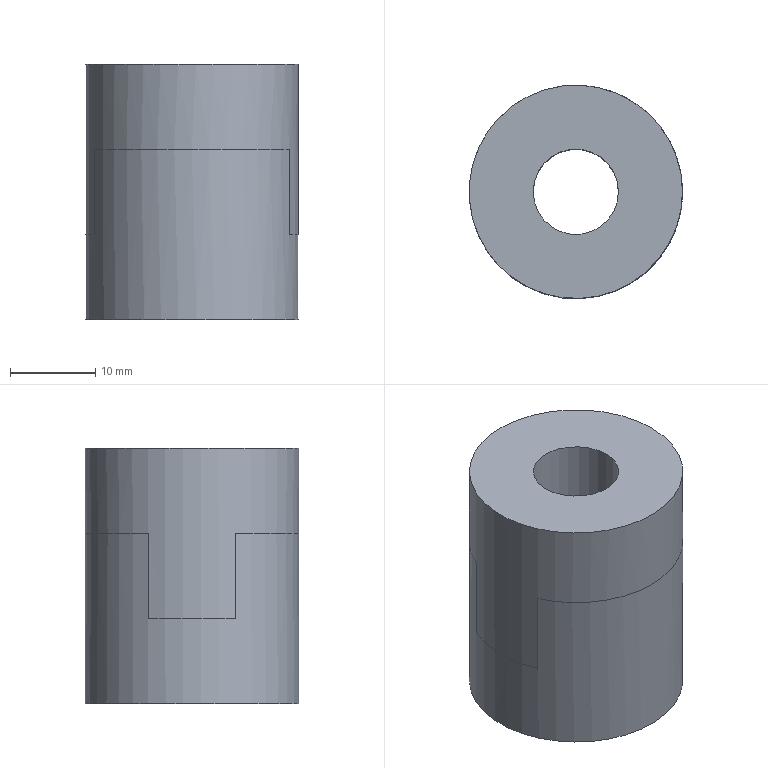Part | NX | features EXTRUDE 6, DATUM_CSYS 4, SKETCH 3 | 2 solids | 16 faces | box 25 x 25 x 30 mm | volume 12370 mm3 | plane 12 | cylinder 4 | commonest cylinder face diameters 10 x2 25 x2
STEP:
#1=CARTESIAN_POINT('',(5.,0.,10.));
#2=VERTEX_POINT('',#1);
#3=CARTESIAN_POINT('',(0.,0.,10.));
#4=DIRECTION('',(0.,0.,1.));
#5=DIRECTION('',(1.,0.,0.));
#6=AXIS2_PLACEMENT_3D('',#3,#4,#5);
#7=CIRCLE('',#6,5.);
#8=EDGE_CURVE('',#2,#2,#7,.T.);
#9=ORIENTED_EDGE('',*,*,#8,.F.);
#10=EDGE_LOOP('',(#9));
#11=FACE_BOUND('',#10,.T.);
#12=CARTESIAN_POINT('',(11.412,-5.1,10.));
#13=VERTEX_POINT('',#12);
#14=CARTESIAN_POINT('',(-11.412,-5.1,10.));
#15=VERTEX_POINT('',#14);
#16=CARTESIAN_POINT('',(11.412,-5.1,10.));
#17=DIRECTION('',(-1.,0.,0.));
#18=VECTOR('',#17,1000.);
#19=LINE('',#16,#18);
#20=EDGE_CURVE('',#13,#15,#19,.T.);
#21=ORIENTED_EDGE('',*,*,#20,.F.);
#22=CARTESIAN_POINT('',(11.412,5.1,10.));
#23=VERTEX_POINT('',#22);
#24=CARTESIAN_POINT('',(0.,0.,10.));
#25=DIRECTION('',(0.,0.,1.));
#26=DIRECTION('',(1.,0.,0.));
#27=AXIS2_PLACEMENT_3D('',#24,#25,#26);
#28=CIRCLE('',#27,12.5);
#29=EDGE_CURVE('',#13,#23,#28,.T.);
#30=ORIENTED_EDGE('',*,*,#29,.T.);
#31=CARTESIAN_POINT('',(-11.412,5.1,10.));
#32=VERTEX_POINT('',#31);
#33=CARTESIAN_POINT('',(-11.412,5.1,10.));
#34=DIRECTION('',(1.,0.,0.));
#35=VECTOR('',#34,1000.);
#36=LINE('',#33,#35);
#37=EDGE_CURVE('',#32,#23,#36,.T.);
#38=ORIENTED_EDGE('',*,*,#37,.F.);
#39=CARTESIAN_POINT('',(0.,0.,10.));
#40=DIRECTION('',(0.,0.,1.));
#41=DIRECTION('',(1.,0.,0.));
#42=AXIS2_PLACEMENT_3D('',#39,#40,#41);
#43=CIRCLE('',#42,12.5);
#44=EDGE_CURVE('',#32,#15,#43,.T.);
#45=ORIENTED_EDGE('',*,*,#44,.T.);
#46=EDGE_LOOP('',(#21,#30,#38,#45));
#47=FACE_BOUND('',#46,.T.);
#48=CARTESIAN_POINT('',(0.,0.,10.));
#49=DIRECTION('',(0.,0.,1.));
#50=DIRECTION('',(1.,0.,0.));
#51=AXIS2_PLACEMENT_3D('',#48,#49,#50);
#52=PLANE('',#51);
#53=ADVANCED_FACE('',(#11,#47),#52,.T.);
#54=ORIENTED_EDGE('',*,*,#44,.F.);
#55=CARTESIAN_POINT('',(-11.412,5.1,20.));
#56=VERTEX_POINT('',#55);
#57=CARTESIAN_POINT('',(-11.412,5.1,20.));
#58=DIRECTION('',(0.,0.,-1.));
#59=VECTOR('',#58,1000.);
#60=LINE('',#57,#59);
#61=EDGE_CURVE('',#32,#56,#60,.F.);
#62=ORIENTED_EDGE('',*,*,#61,.T.);
#63=CARTESIAN_POINT('',(11.412,5.1,20.));
#64=VERTEX_POINT('',#63);
#65=CARTESIAN_POINT('',(0.,0.,20.));
#66=DIRECTION('',(0.,0.,1.));
#67=DIRECTION('',(1.,0.,0.));
#68=AXIS2_PLACEMENT_3D('',#65,#66,#67);
#69=CIRCLE('',#68,12.5);
#70=EDGE_CURVE('',#64,#56,#69,.T.);
#71=ORIENTED_EDGE('',*,*,#70,.F.);
#72=CARTESIAN_POINT('',(11.412,5.1,20.));
#73=DIRECTION('',(0.,0.,-1.));
#74=VECTOR('',#73,1000.);
#75=LINE('',#72,#74);
#76=EDGE_CURVE('',#64,#23,#75,.T.);
#77=ORIENTED_EDGE('',*,*,#76,.T.);
#78=ORIENTED_EDGE('',*,*,#29,.F.);
#79=CARTESIAN_POINT('',(11.412,-5.1,20.));
#80=VERTEX_POINT('',#79);
#81=CARTESIAN_POINT('',(11.412,-5.1,20.));
#82=DIRECTION('',(0.,0.,-1.));
#83=VECTOR('',#82,1000.);
#84=LINE('',#81,#83);
#85=EDGE_CURVE('',#13,#80,#84,.F.);
#86=ORIENTED_EDGE('',*,*,#85,.T.);
#87=CARTESIAN_POINT('',(-11.412,-5.1,20.));
#88=VERTEX_POINT('',#87);
#89=CARTESIAN_POINT('',(0.,0.,20.));
#90=DIRECTION('',(0.,0.,1.));
#91=DIRECTION('',(1.,0.,0.));
#92=AXIS2_PLACEMENT_3D('',#89,#90,#91);
#93=CIRCLE('',#92,12.5);
#94=EDGE_CURVE('',#88,#80,#93,.T.);
#95=ORIENTED_EDGE('',*,*,#94,.F.);
#96=CARTESIAN_POINT('',(-11.412,-5.1,20.));
#97=DIRECTION('',(0.,0.,-1.));
#98=VECTOR('',#97,1000.);
#99=LINE('',#96,#98);
#100=EDGE_CURVE('',#88,#15,#99,.T.);
#101=ORIENTED_EDGE('',*,*,#100,.T.);
#102=EDGE_LOOP('',(#54,#62,#71,#77,#78,#86,#95,#101));
#103=FACE_BOUND('',#102,.T.);
#104=CARTESIAN_POINT('',(12.5,0.,0.));
#105=VERTEX_POINT('',#104);
#106=CARTESIAN_POINT('',(0.,0.,0.));
#107=DIRECTION('',(0.,0.,1.));
#108=DIRECTION('',(1.,0.,0.));
#109=AXIS2_PLACEMENT_3D('',#106,#107,#108);
#110=CIRCLE('',#109,12.5);
#111=EDGE_CURVE('',#105,#105,#110,.T.);
#112=ORIENTED_EDGE('',*,*,#111,.T.);
#113=EDGE_LOOP('',(#112));
#114=FACE_BOUND('',#113,.T.);
#115=CARTESIAN_POINT('',(0.,0.,10.));
#116=DIRECTION('',(0.,0.,-1.));
#117=DIRECTION('',(-1.,0.,0.));
#118=AXIS2_PLACEMENT_3D('',#115,#116,#117);
#119=CYLINDRICAL_SURFACE('',#118,12.5);
#120=ADVANCED_FACE('',(#103,#114),#119,.T.);
#121=CARTESIAN_POINT('',(5.,0.,0.));
#122=VERTEX_POINT('',#121);
#123=CARTESIAN_POINT('',(0.,0.,0.));
#124=DIRECTION('',(0.,0.,1.));
#125=DIRECTION('',(1.,0.,0.));
#126=AXIS2_PLACEMENT_3D('',#123,#124,#125);
#127=CIRCLE('',#126,5.);
#128=EDGE_CURVE('',#122,#122,#127,.T.);
#129=ORIENTED_EDGE('',*,*,#128,.T.);
#130=EDGE_LOOP('',(#129));
#131=FACE_BOUND('',#130,.T.);
#132=ORIENTED_EDGE('',*,*,#111,.F.);
#133=EDGE_LOOP('',(#132));
#134=FACE_BOUND('',#133,.T.);
#135=CARTESIAN_POINT('',(0.,0.,0.));
#136=DIRECTION('',(0.,0.,1.));
#137=DIRECTION('',(1.,0.,0.));
#138=AXIS2_PLACEMENT_3D('',#135,#136,#137);
#139=PLANE('',#138);
#140=ADVANCED_FACE('',(#131,#134),#139,.F.);
#141=ORIENTED_EDGE('',*,*,#37,.T.);
#142=ORIENTED_EDGE('',*,*,#76,.F.);
#143=CARTESIAN_POINT('',(-11.412,5.1,20.));
#144=DIRECTION('',(1.,0.,0.));
#145=VECTOR('',#144,1000.);
#146=LINE('',#143,#145);
#147=EDGE_CURVE('',#56,#64,#146,.T.);
#148=ORIENTED_EDGE('',*,*,#147,.F.);
#149=ORIENTED_EDGE('',*,*,#61,.F.);
#150=EDGE_LOOP('',(#141,#142,#148,#149));
#151=FACE_BOUND('',#150,.T.);
#152=CARTESIAN_POINT('',(-11.412,5.1,20.));
#153=DIRECTION('',(0.,1.,0.));
#154=DIRECTION('',(0.,0.,1.));
#155=AXIS2_PLACEMENT_3D('',#152,#153,#154);
#156=PLANE('',#155);
#157=ADVANCED_FACE('',(#151),#156,.F.);
#158=ORIENTED_EDGE('',*,*,#147,.T.);
#159=ORIENTED_EDGE('',*,*,#70,.T.);
#160=EDGE_LOOP('',(#158,#159));
#161=FACE_BOUND('',#160,.T.);
#162=CARTESIAN_POINT('',(0.,0.,20.));
#163=DIRECTION('',(0.,0.,1.));
#164=DIRECTION('',(1.,0.,0.));
#165=AXIS2_PLACEMENT_3D('',#162,#163,#164);
#166=PLANE('',#165);
#167=ADVANCED_FACE('',(#161),#166,.T.);
#168=ORIENTED_EDGE('',*,*,#20,.T.);
#169=ORIENTED_EDGE('',*,*,#100,.F.);
#170=CARTESIAN_POINT('',(11.412,-5.1,20.));
#171=DIRECTION('',(-1.,0.,0.));
#172=VECTOR('',#171,1000.);
#173=LINE('',#170,#172);
#174=EDGE_CURVE('',#80,#88,#173,.T.);
#175=ORIENTED_EDGE('',*,*,#174,.F.);
#176=ORIENTED_EDGE('',*,*,#85,.F.);
#177=EDGE_LOOP('',(#168,#169,#175,#176));
#178=FACE_BOUND('',#177,.T.);
#179=CARTESIAN_POINT('',(11.412,-5.1,20.));
#180=DIRECTION('',(0.,-1.,0.));
#181=DIRECTION('',(0.,0.,-1.));
#182=AXIS2_PLACEMENT_3D('',#179,#180,#181);
#183=PLANE('',#182);
#184=ADVANCED_FACE('',(#178),#183,.F.);
#185=ORIENTED_EDGE('',*,*,#174,.T.);
#186=ORIENTED_EDGE('',*,*,#94,.T.);
#187=EDGE_LOOP('',(#185,#186));
#188=FACE_BOUND('',#187,.T.);
#189=CARTESIAN_POINT('',(0.,0.,20.));
#190=DIRECTION('',(0.,0.,1.));
#191=DIRECTION('',(1.,0.,0.));
#192=AXIS2_PLACEMENT_3D('',#189,#190,#191);
#193=PLANE('',#192);
#194=ADVANCED_FACE('',(#188),#193,.T.);
#195=ORIENTED_EDGE('',*,*,#8,.T.);
#196=EDGE_LOOP('',(#195));
#197=FACE_BOUND('',#196,.T.);
#198=ORIENTED_EDGE('',*,*,#128,.F.);
#199=EDGE_LOOP('',(#198));
#200=FACE_BOUND('',#199,.T.);
#201=CARTESIAN_POINT('',(0.,0.,-30.));
#202=DIRECTION('',(0.,0.,1.));
#203=DIRECTION('',(1.,0.,0.));
#204=AXIS2_PLACEMENT_3D('',#201,#202,#203);
#205=CYLINDRICAL_SURFACE('',#204,5.);
#206=ADVANCED_FACE('',(#197,#200),#205,.F.);
#207=CLOSED_SHELL('',(#53,#120,#140,#157,#167,#184,#194,#206));
#208=MANIFOLD_SOLID_BREP('',#207);
#209=CARTESIAN_POINT('',(11.412,5.1,10.));
#210=VERTEX_POINT('',#209);
#211=CARTESIAN_POINT('',(-11.412,5.1,10.));
#212=VERTEX_POINT('',#211);
#213=CARTESIAN_POINT('',(11.412,5.1,10.));
#214=DIRECTION('',(-1.,0.,0.));
#215=VECTOR('',#214,1000.);
#216=LINE('',#213,#215);
#217=EDGE_CURVE('',#210,#212,#216,.T.);
#218=ORIENTED_EDGE('',*,*,#217,.T.);
#219=CARTESIAN_POINT('',(-11.412,5.1,20.));
#220=VERTEX_POINT('',#219);
#221=CARTESIAN_POINT('',(-11.412,5.1,20.));
#222=DIRECTION('',(0.,0.,-1.));
#223=VECTOR('',#222,1000.);
#224=LINE('',#221,#223);
#225=EDGE_CURVE('',#212,#220,#224,.F.);
#226=ORIENTED_EDGE('',*,*,#225,.T.);
#227=CARTESIAN_POINT('',(11.412,5.1,20.));
#228=VERTEX_POINT('',#227);
#229=CARTESIAN_POINT('',(11.412,5.1,20.));
#230=DIRECTION('',(-1.,0.,0.));
#231=VECTOR('',#230,1000.);
#232=LINE('',#229,#231);
#233=EDGE_CURVE('',#228,#220,#232,.T.);
#234=ORIENTED_EDGE('',*,*,#233,.F.);
#235=CARTESIAN_POINT('',(11.412,5.1,20.));
#236=DIRECTION('',(0.,0.,-1.));
#237=VECTOR('',#236,1000.);
#238=LINE('',#235,#237);
#239=EDGE_CURVE('',#228,#210,#238,.T.);
#240=ORIENTED_EDGE('',*,*,#239,.T.);
#241=EDGE_LOOP('',(#218,#226,#234,#240));
#242=FACE_BOUND('',#241,.T.);
#243=CARTESIAN_POINT('',(11.412,5.1,20.));
#244=DIRECTION('',(0.,-1.,0.));
#245=DIRECTION('',(0.,0.,-1.));
#246=AXIS2_PLACEMENT_3D('',#243,#244,#245);
#247=PLANE('',#246);
#248=ADVANCED_FACE('',(#242),#247,.F.);
#249=CARTESIAN_POINT('',(-11.412,-5.1,10.));
#250=VERTEX_POINT('',#249);
#251=CARTESIAN_POINT('',(0.,0.,10.));
#252=DIRECTION('',(0.,0.,1.));
#253=DIRECTION('',(1.,0.,0.));
#254=AXIS2_PLACEMENT_3D('',#251,#252,#253);
#255=CIRCLE('',#254,12.5);
#256=EDGE_CURVE('',#212,#250,#255,.T.);
#257=ORIENTED_EDGE('',*,*,#256,.T.);
#258=CARTESIAN_POINT('',(-11.412,-5.1,20.));
#259=VERTEX_POINT('',#258);
#260=CARTESIAN_POINT('',(-11.412,-5.1,20.));
#261=DIRECTION('',(0.,0.,-1.));
#262=VECTOR('',#261,1000.);
#263=LINE('',#260,#262);
#264=EDGE_CURVE('',#250,#259,#263,.F.);
#265=ORIENTED_EDGE('',*,*,#264,.T.);
#266=CARTESIAN_POINT('',(11.412,-5.1,20.));
#267=VERTEX_POINT('',#266);
#268=CARTESIAN_POINT('',(0.,0.,20.));
#269=DIRECTION('',(0.,0.,-1.));
#270=DIRECTION('',(1.,0.,0.));
#271=AXIS2_PLACEMENT_3D('',#268,#269,#270);
#272=CIRCLE('',#271,12.5);
#273=EDGE_CURVE('',#267,#259,#272,.T.);
#274=ORIENTED_EDGE('',*,*,#273,.F.);
#275=CARTESIAN_POINT('',(11.412,-5.1,10.));
#276=VERTEX_POINT('',#275);
#277=CARTESIAN_POINT('',(11.412,-5.1,20.));
#278=DIRECTION('',(0.,0.,-1.));
#279=VECTOR('',#278,1000.);
#280=LINE('',#277,#279);
#281=EDGE_CURVE('',#267,#276,#280,.T.);
#282=ORIENTED_EDGE('',*,*,#281,.T.);
#283=CARTESIAN_POINT('',(0.,0.,10.));
#284=DIRECTION('',(0.,0.,1.));
#285=DIRECTION('',(1.,0.,0.));
#286=AXIS2_PLACEMENT_3D('',#283,#284,#285);
#287=CIRCLE('',#286,12.5);
#288=EDGE_CURVE('',#276,#210,#287,.T.);
#289=ORIENTED_EDGE('',*,*,#288,.T.);
#290=ORIENTED_EDGE('',*,*,#239,.F.);
#291=CARTESIAN_POINT('',(0.,0.,20.));
#292=DIRECTION('',(0.,0.,-1.));
#293=DIRECTION('',(1.,0.,0.));
#294=AXIS2_PLACEMENT_3D('',#291,#292,#293);
#295=CIRCLE('',#294,12.5);
#296=EDGE_CURVE('',#220,#228,#295,.T.);
#297=ORIENTED_EDGE('',*,*,#296,.F.);
#298=ORIENTED_EDGE('',*,*,#225,.F.);
#299=EDGE_LOOP('',(#257,#265,#274,#282,#289,#290,#297,#298));
#300=FACE_BOUND('',#299,.T.);
#301=CARTESIAN_POINT('',(12.5,0.,30.));
#302=VERTEX_POINT('',#301);
#303=CARTESIAN_POINT('',(0.,0.,30.));
#304=DIRECTION('',(0.,0.,-1.));
#305=DIRECTION('',(1.,0.,0.));
#306=AXIS2_PLACEMENT_3D('',#303,#304,#305);
#307=CIRCLE('',#306,12.5);
#308=EDGE_CURVE('',#302,#302,#307,.T.);
#309=ORIENTED_EDGE('',*,*,#308,.T.);
#310=EDGE_LOOP('',(#309));
#311=FACE_BOUND('',#310,.T.);
#312=CARTESIAN_POINT('',(0.,0.,20.));
#313=DIRECTION('',(0.,0.,-1.));
#314=DIRECTION('',(-1.,0.,0.));
#315=AXIS2_PLACEMENT_3D('',#312,#313,#314);
#316=CYLINDRICAL_SURFACE('',#315,12.5);
#317=ADVANCED_FACE('',(#300,#311),#316,.T.);
#318=CARTESIAN_POINT('',(-11.412,-5.1,10.));
#319=DIRECTION('',(1.,0.,0.));
#320=VECTOR('',#319,1000.);
#321=LINE('',#318,#320);
#322=EDGE_CURVE('',#250,#276,#321,.T.);
#323=ORIENTED_EDGE('',*,*,#322,.T.);
#324=ORIENTED_EDGE('',*,*,#281,.F.);
#325=CARTESIAN_POINT('',(-11.412,-5.1,20.));
#326=DIRECTION('',(1.,0.,0.));
#327=VECTOR('',#326,1000.);
#328=LINE('',#325,#327);
#329=EDGE_CURVE('',#259,#267,#328,.T.);
#330=ORIENTED_EDGE('',*,*,#329,.F.);
#331=ORIENTED_EDGE('',*,*,#264,.F.);
#332=EDGE_LOOP('',(#323,#324,#330,#331));
#333=FACE_BOUND('',#332,.T.);
#334=CARTESIAN_POINT('',(-11.412,-5.1,20.));
#335=DIRECTION('',(0.,1.,0.));
#336=DIRECTION('',(0.,0.,1.));
#337=AXIS2_PLACEMENT_3D('',#334,#335,#336);
#338=PLANE('',#337);
#339=ADVANCED_FACE('',(#333),#338,.F.);
#340=CARTESIAN_POINT('',(5.,0.,10.));
#341=VERTEX_POINT('',#340);
#342=CARTESIAN_POINT('',(0.,0.,10.));
#343=DIRECTION('',(0.,0.,1.));
#344=DIRECTION('',(1.,0.,0.));
#345=AXIS2_PLACEMENT_3D('',#342,#343,#344);
#346=CIRCLE('',#345,5.);
#347=EDGE_CURVE('',#341,#341,#346,.T.);
#348=ORIENTED_EDGE('',*,*,#347,.T.);
#349=EDGE_LOOP('',(#348));
#350=FACE_BOUND('',#349,.T.);
#351=ORIENTED_EDGE('',*,*,#288,.F.);
#352=ORIENTED_EDGE('',*,*,#322,.F.);
#353=ORIENTED_EDGE('',*,*,#256,.F.);
#354=ORIENTED_EDGE('',*,*,#217,.F.);
#355=EDGE_LOOP('',(#351,#352,#353,#354));
#356=FACE_BOUND('',#355,.T.);
#357=CARTESIAN_POINT('',(0.,0.,10.));
#358=DIRECTION('',(0.,0.,1.));
#359=DIRECTION('',(1.,0.,0.));
#360=AXIS2_PLACEMENT_3D('',#357,#358,#359);
#361=PLANE('',#360);
#362=ADVANCED_FACE('',(#350,#356),#361,.F.);
#363=ORIENTED_EDGE('',*,*,#296,.T.);
#364=ORIENTED_EDGE('',*,*,#233,.T.);
#365=EDGE_LOOP('',(#363,#364));
#366=FACE_BOUND('',#365,.T.);
#367=CARTESIAN_POINT('',(0.,0.,20.));
#368=DIRECTION('',(0.,0.,-1.));
#369=DIRECTION('',(-1.,0.,0.));
#370=AXIS2_PLACEMENT_3D('',#367,#368,#369);
#371=PLANE('',#370);
#372=ADVANCED_FACE('',(#366),#371,.T.);
#373=CARTESIAN_POINT('',(5.,0.,30.));
#374=VERTEX_POINT('',#373);
#375=CARTESIAN_POINT('',(0.,0.,30.));
#376=DIRECTION('',(0.,0.,1.));
#377=DIRECTION('',(1.,0.,0.));
#378=AXIS2_PLACEMENT_3D('',#375,#376,#377);
#379=CIRCLE('',#378,5.);
#380=EDGE_CURVE('',#374,#374,#379,.T.);
#381=ORIENTED_EDGE('',*,*,#380,.F.);
#382=EDGE_LOOP('',(#381));
#383=FACE_BOUND('',#382,.T.);
#384=ORIENTED_EDGE('',*,*,#308,.F.);
#385=EDGE_LOOP('',(#384));
#386=FACE_BOUND('',#385,.T.);
#387=CARTESIAN_POINT('',(0.,0.,30.));
#388=DIRECTION('',(0.,0.,-1.));
#389=DIRECTION('',(-1.,0.,0.));
#390=AXIS2_PLACEMENT_3D('',#387,#388,#389);
#391=PLANE('',#390);
#392=ADVANCED_FACE('',(#383,#386),#391,.F.);
#393=ORIENTED_EDGE('',*,*,#273,.T.);
#394=ORIENTED_EDGE('',*,*,#329,.T.);
#395=EDGE_LOOP('',(#393,#394));
#396=FACE_BOUND('',#395,.T.);
#397=CARTESIAN_POINT('',(0.,0.,20.));
#398=DIRECTION('',(0.,0.,-1.));
#399=DIRECTION('',(-1.,0.,0.));
#400=AXIS2_PLACEMENT_3D('',#397,#398,#399);
#401=PLANE('',#400);
#402=ADVANCED_FACE('',(#396),#401,.T.);
#403=ORIENTED_EDGE('',*,*,#380,.T.);
#404=EDGE_LOOP('',(#403));
#405=FACE_BOUND('',#404,.T.);
#406=ORIENTED_EDGE('',*,*,#347,.F.);
#407=EDGE_LOOP('',(#406));
#408=FACE_BOUND('',#407,.T.);
#409=CARTESIAN_POINT('',(0.,0.,-30.));
#410=DIRECTION('',(0.,0.,1.));
#411=DIRECTION('',(1.,0.,0.));
#412=AXIS2_PLACEMENT_3D('',#409,#410,#411);
#413=CYLINDRICAL_SURFACE('',#412,5.);
#414=ADVANCED_FACE('',(#405,#408),#413,.F.);
#415=CLOSED_SHELL('',(#248,#317,#339,#362,#372,#392,#402,#414));
#416=MANIFOLD_SOLID_BREP('',#415);
#417=(LENGTH_UNIT()NAMED_UNIT(*)SI_UNIT(.MILLI.,.METRE.));
#418=UNCERTAINTY_MEASURE_WITH_UNIT(LENGTH_MEASURE(0.00001),#417,'','');
#419=(NAMED_UNIT(*)PLANE_ANGLE_UNIT()SI_UNIT($,.RADIAN.));
#420=(NAMED_UNIT(*)SI_UNIT($,.STERADIAN.)SOLID_ANGLE_UNIT());
#421=(GEOMETRIC_REPRESENTATION_CONTEXT(3)GLOBAL_UNCERTAINTY_ASSIGNED_CONTEXT((#418))GLOBAL_UNIT_ASSIGNED_CONTEXT((#417,#419,#420))REPRESENTATION_CONTEXT('',''));
#422=ADVANCED_BREP_SHAPE_REPRESENTATION('',(#208,#416),#421);